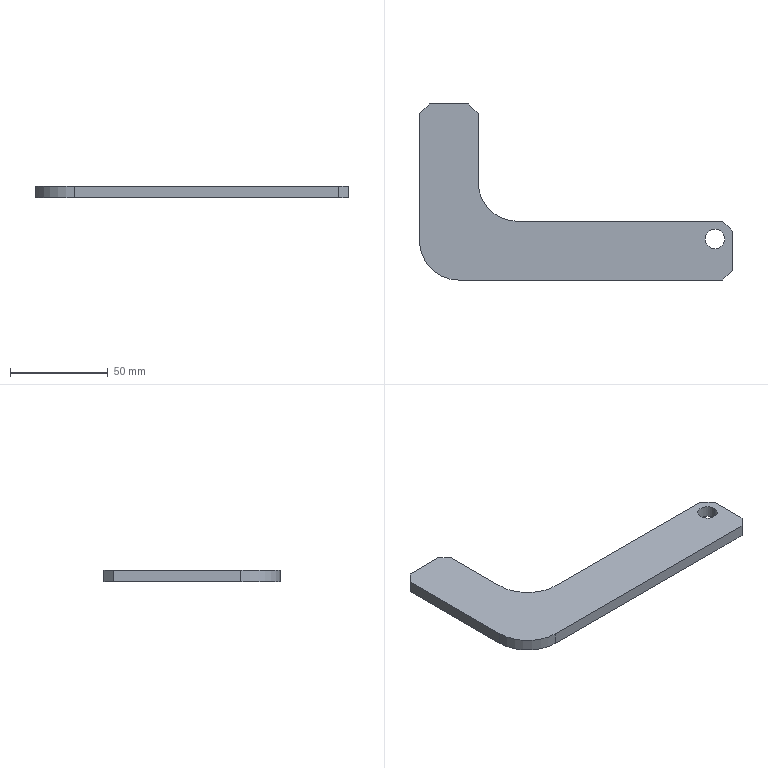Part | STEP file | [02]-12 | 1 solid | 16 faces | box 160 x 90 x 6 mm | volume 38829 mm3 | plane 12 | cylinder 4 | commonest cylinder face diameters 10 x2 40 x2
STEP:
#1=CARTESIAN_POINT('',(146.,21.,6.));
#2=VERTEX_POINT('',#1);
#3=CARTESIAN_POINT('',(156.,21.,6.));
#4=VERTEX_POINT('',#3);
#5=CARTESIAN_POINT('',(151.,21.,6.));
#6=DIRECTION('',(0.,0.,-1.));
#7=DIRECTION('',(1.,0.,0.));
#8=AXIS2_PLACEMENT_3D('',#5,#6,#7);
#9=CIRCLE('',#8,5.);
#10=EDGE_CURVE('',#2,#4,#9,.T.);
#11=ORIENTED_EDGE('',*,*,#10,.F.);
#12=CARTESIAN_POINT('',(146.,21.,0.));
#13=VERTEX_POINT('',#12);
#14=CARTESIAN_POINT('',(146.,21.,6.));
#15=DIRECTION('',(0.,0.,-1.));
#16=VECTOR('',#15,1000.);
#17=LINE('',#14,#16);
#18=EDGE_CURVE('',#2,#13,#17,.T.);
#19=ORIENTED_EDGE('',*,*,#18,.T.);
#20=CARTESIAN_POINT('',(156.,21.,0.));
#21=VERTEX_POINT('',#20);
#22=CARTESIAN_POINT('',(151.,21.,0.));
#23=DIRECTION('',(0.,0.,1.));
#24=DIRECTION('',(-1.,0.,0.));
#25=AXIS2_PLACEMENT_3D('',#22,#23,#24);
#26=CIRCLE('',#25,5.);
#27=EDGE_CURVE('',#21,#13,#26,.T.);
#28=ORIENTED_EDGE('',*,*,#27,.F.);
#29=CARTESIAN_POINT('',(156.,21.,6.));
#30=DIRECTION('',(0.,0.,-1.));
#31=VECTOR('',#30,1000.);
#32=LINE('',#29,#31);
#33=EDGE_CURVE('',#4,#21,#32,.T.);
#34=ORIENTED_EDGE('',*,*,#33,.F.);
#35=EDGE_LOOP('',(#11,#19,#28,#34));
#36=FACE_OUTER_BOUND('',#35,.T.);
#37=CARTESIAN_POINT('',(151.,21.,6.));
#38=DIRECTION('',(0.,0.,-1.));
#39=DIRECTION('',(1.,0.,0.));
#40=AXIS2_PLACEMENT_3D('',#37,#38,#39);
#41=CYLINDRICAL_SURFACE('',#40,5.);
#42=ADVANCED_FACE('',(#36),#41,.F.);
#43=CARTESIAN_POINT('',(50.,30.,6.));
#44=VERTEX_POINT('',#43);
#45=CARTESIAN_POINT('',(155.,30.,6.));
#46=VERTEX_POINT('',#45);
#47=CARTESIAN_POINT('',(80.,30.,6.));
#48=DIRECTION('',(1.,0.,0.));
#49=VECTOR('',#48,1000.);
#50=LINE('',#47,#49);
#51=EDGE_CURVE('',#44,#46,#50,.T.);
#52=ORIENTED_EDGE('',*,*,#51,.T.);
#53=CARTESIAN_POINT('',(155.,30.,0.));
#54=VERTEX_POINT('',#53);
#55=CARTESIAN_POINT('',(155.,30.,0.));
#56=DIRECTION('',(0.,0.,-1.));
#57=VECTOR('',#56,1000.);
#58=LINE('',#55,#57);
#59=EDGE_CURVE('',#46,#54,#58,.T.);
#60=ORIENTED_EDGE('',*,*,#59,.T.);
#61=CARTESIAN_POINT('',(50.,30.,0.));
#62=VERTEX_POINT('',#61);
#63=CARTESIAN_POINT('',(80.,30.,0.));
#64=DIRECTION('',(-1.,0.,0.));
#65=VECTOR('',#64,1000.);
#66=LINE('',#63,#65);
#67=EDGE_CURVE('',#54,#62,#66,.T.);
#68=ORIENTED_EDGE('',*,*,#67,.T.);
#69=CARTESIAN_POINT('',(50.,30.,6.));
#70=DIRECTION('',(0.,0.,1.));
#71=VECTOR('',#70,1000.);
#72=LINE('',#69,#71);
#73=EDGE_CURVE('',#62,#44,#72,.T.);
#74=ORIENTED_EDGE('',*,*,#73,.T.);
#75=EDGE_LOOP('',(#52,#60,#68,#74));
#76=FACE_OUTER_BOUND('',#75,.T.);
#77=CARTESIAN_POINT('',(80.,30.,0.));
#78=DIRECTION('',(0.,1.,0.));
#79=DIRECTION('',(0.,0.,1.));
#80=AXIS2_PLACEMENT_3D('',#77,#78,#79);
#81=PLANE('',#80);
#82=ADVANCED_FACE('',(#76),#81,.T.);
#83=CARTESIAN_POINT('',(151.,21.,6.));
#84=DIRECTION('',(0.,0.,-1.));
#85=DIRECTION('',(1.,0.,0.));
#86=AXIS2_PLACEMENT_3D('',#83,#84,#85);
#87=CIRCLE('',#86,5.);
#88=EDGE_CURVE('',#4,#2,#87,.T.);
#89=ORIENTED_EDGE('',*,*,#88,.T.);
#90=ORIENTED_EDGE('',*,*,#10,.T.);
#91=EDGE_LOOP('',(#89,#90));
#92=FACE_BOUND('',#91,.T.);
#93=CARTESIAN_POINT('',(0.,20.,6.));
#94=VERTEX_POINT('',#93);
#95=CARTESIAN_POINT('',(0.,85.,6.));
#96=VERTEX_POINT('',#95);
#97=CARTESIAN_POINT('',(0.,15.,6.));
#98=DIRECTION('',(0.,1.,0.));
#99=VECTOR('',#98,1000.);
#100=LINE('',#97,#99);
#101=EDGE_CURVE('',#94,#96,#100,.T.);
#102=ORIENTED_EDGE('',*,*,#101,.F.);
#103=CARTESIAN_POINT('',(20.,0.,6.));
#104=VERTEX_POINT('',#103);
#105=CARTESIAN_POINT('',(20.,20.,6.));
#106=DIRECTION('',(0.,0.,1.));
#107=DIRECTION('',(0.,-1.,0.));
#108=AXIS2_PLACEMENT_3D('',#105,#106,#107);
#109=CIRCLE('',#108,20.);
#110=EDGE_CURVE('',#94,#104,#109,.T.);
#111=ORIENTED_EDGE('',*,*,#110,.T.);
#112=CARTESIAN_POINT('',(155.,0.,6.));
#113=VERTEX_POINT('',#112);
#114=CARTESIAN_POINT('',(80.,0.,6.));
#115=DIRECTION('',(-1.,0.,0.));
#116=VECTOR('',#115,1000.);
#117=LINE('',#114,#116);
#118=EDGE_CURVE('',#113,#104,#117,.T.);
#119=ORIENTED_EDGE('',*,*,#118,.F.);
#120=CARTESIAN_POINT('',(160.,5.,6.));
#121=VERTEX_POINT('',#120);
#122=CARTESIAN_POINT('',(125.,-30.,6.));
#123=DIRECTION('',(0.7071,0.7071,0.));
#124=VECTOR('',#123,1000.);
#125=LINE('',#122,#124);
#126=EDGE_CURVE('',#113,#121,#125,.T.);
#127=ORIENTED_EDGE('',*,*,#126,.T.);
#128=CARTESIAN_POINT('',(160.,25.,6.));
#129=VERTEX_POINT('',#128);
#130=CARTESIAN_POINT('',(160.,15.,6.));
#131=DIRECTION('',(0.,-1.,0.));
#132=VECTOR('',#131,1000.);
#133=LINE('',#130,#132);
#134=EDGE_CURVE('',#129,#121,#133,.T.);
#135=ORIENTED_EDGE('',*,*,#134,.F.);
#136=CARTESIAN_POINT('',(125.,60.,6.));
#137=DIRECTION('',(-0.7071,0.7071,0.));
#138=VECTOR('',#137,1000.);
#139=LINE('',#136,#138);
#140=EDGE_CURVE('',#129,#46,#139,.T.);
#141=ORIENTED_EDGE('',*,*,#140,.T.);
#142=ORIENTED_EDGE('',*,*,#51,.F.);
#143=CARTESIAN_POINT('',(30.,50.,6.));
#144=VERTEX_POINT('',#143);
#145=CARTESIAN_POINT('',(50.,50.,6.));
#146=DIRECTION('',(0.,0.,-1.));
#147=DIRECTION('',(0.,-1.,0.));
#148=AXIS2_PLACEMENT_3D('',#145,#146,#147);
#149=CIRCLE('',#148,20.);
#150=EDGE_CURVE('',#44,#144,#149,.T.);
#151=ORIENTED_EDGE('',*,*,#150,.T.);
#152=CARTESIAN_POINT('',(30.,85.,6.));
#153=VERTEX_POINT('',#152);
#154=CARTESIAN_POINT('',(30.,60.,6.));
#155=DIRECTION('',(0.,-1.,0.));
#156=VECTOR('',#155,1000.);
#157=LINE('',#154,#156);
#158=EDGE_CURVE('',#153,#144,#157,.T.);
#159=ORIENTED_EDGE('',*,*,#158,.F.);
#160=CARTESIAN_POINT('',(25.,90.,6.));
#161=VERTEX_POINT('',#160);
#162=CARTESIAN_POINT('',(90.,25.,6.));
#163=DIRECTION('',(-0.7071,0.7071,0.));
#164=VECTOR('',#163,1000.);
#165=LINE('',#162,#164);
#166=EDGE_CURVE('',#153,#161,#165,.T.);
#167=ORIENTED_EDGE('',*,*,#166,.T.);
#168=CARTESIAN_POINT('',(5.,90.,6.));
#169=VERTEX_POINT('',#168);
#170=CARTESIAN_POINT('',(15.,90.,6.));
#171=DIRECTION('',(1.,0.,0.));
#172=VECTOR('',#171,1000.);
#173=LINE('',#170,#172);
#174=EDGE_CURVE('',#169,#161,#173,.T.);
#175=ORIENTED_EDGE('',*,*,#174,.F.);
#176=CARTESIAN_POINT('',(5.,90.,6.));
#177=DIRECTION('',(-0.7071,-0.7071,0.));
#178=VECTOR('',#177,1000.);
#179=LINE('',#176,#178);
#180=EDGE_CURVE('',#169,#96,#179,.T.);
#181=ORIENTED_EDGE('',*,*,#180,.T.);
#182=EDGE_LOOP('',(#102,#111,#119,#127,#135,#141,#142,#151,#159,#167,#175,#181));
#183=FACE_OUTER_BOUND('',#182,.T.);
#184=CARTESIAN_POINT('',(80.,15.,6.));
#185=DIRECTION('',(0.,0.,1.));
#186=DIRECTION('',(0.,-1.,0.));
#187=AXIS2_PLACEMENT_3D('',#184,#185,#186);
#188=PLANE('',#187);
#189=ADVANCED_FACE('',(#92,#183),#188,.T.);
#190=CARTESIAN_POINT('',(0.,85.,0.));
#191=VERTEX_POINT('',#190);
#192=CARTESIAN_POINT('',(0.,20.,0.));
#193=VERTEX_POINT('',#192);
#194=CARTESIAN_POINT('',(0.,15.,0.));
#195=DIRECTION('',(0.,-1.,0.));
#196=VECTOR('',#195,1000.);
#197=LINE('',#194,#196);
#198=EDGE_CURVE('',#191,#193,#197,.T.);
#199=ORIENTED_EDGE('',*,*,#198,.T.);
#200=CARTESIAN_POINT('',(0.,20.,0.));
#201=DIRECTION('',(0.,0.,1.));
#202=VECTOR('',#201,1000.);
#203=LINE('',#200,#202);
#204=EDGE_CURVE('',#193,#94,#203,.T.);
#205=ORIENTED_EDGE('',*,*,#204,.T.);
#206=ORIENTED_EDGE('',*,*,#101,.T.);
#207=CARTESIAN_POINT('',(0.,85.,0.));
#208=DIRECTION('',(0.,0.,-1.));
#209=VECTOR('',#208,1000.);
#210=LINE('',#207,#209);
#211=EDGE_CURVE('',#96,#191,#210,.T.);
#212=ORIENTED_EDGE('',*,*,#211,.T.);
#213=EDGE_LOOP('',(#199,#205,#206,#212));
#214=FACE_OUTER_BOUND('',#213,.T.);
#215=CARTESIAN_POINT('',(0.,15.,0.));
#216=DIRECTION('',(-1.,0.,0.));
#217=DIRECTION('',(0.,0.,-1.));
#218=AXIS2_PLACEMENT_3D('',#215,#216,#217);
#219=PLANE('',#218);
#220=ADVANCED_FACE('',(#214),#219,.T.);
#221=CARTESIAN_POINT('',(160.,5.,0.));
#222=VERTEX_POINT('',#221);
#223=CARTESIAN_POINT('',(160.,25.,0.));
#224=VERTEX_POINT('',#223);
#225=CARTESIAN_POINT('',(160.,15.,0.));
#226=DIRECTION('',(0.,1.,0.));
#227=VECTOR('',#226,1000.);
#228=LINE('',#225,#227);
#229=EDGE_CURVE('',#222,#224,#228,.T.);
#230=ORIENTED_EDGE('',*,*,#229,.T.);
#231=CARTESIAN_POINT('',(160.,25.,0.));
#232=DIRECTION('',(0.,0.,1.));
#233=VECTOR('',#232,1000.);
#234=LINE('',#231,#233);
#235=EDGE_CURVE('',#224,#129,#234,.T.);
#236=ORIENTED_EDGE('',*,*,#235,.T.);
#237=ORIENTED_EDGE('',*,*,#134,.T.);
#238=CARTESIAN_POINT('',(160.,5.,0.));
#239=DIRECTION('',(0.,0.,-1.));
#240=VECTOR('',#239,1000.);
#241=LINE('',#238,#240);
#242=EDGE_CURVE('',#121,#222,#241,.T.);
#243=ORIENTED_EDGE('',*,*,#242,.T.);
#244=EDGE_LOOP('',(#230,#236,#237,#243));
#245=FACE_OUTER_BOUND('',#244,.T.);
#246=CARTESIAN_POINT('',(160.,15.,0.));
#247=DIRECTION('',(1.,0.,0.));
#248=DIRECTION('',(0.,0.,1.));
#249=AXIS2_PLACEMENT_3D('',#246,#247,#248);
#250=PLANE('',#249);
#251=ADVANCED_FACE('',(#245),#250,.T.);
#252=ORIENTED_EDGE('',*,*,#27,.T.);
#253=CARTESIAN_POINT('',(151.,21.,0.));
#254=DIRECTION('',(0.,0.,1.));
#255=DIRECTION('',(-1.,0.,0.));
#256=AXIS2_PLACEMENT_3D('',#253,#254,#255);
#257=CIRCLE('',#256,5.);
#258=EDGE_CURVE('',#13,#21,#257,.T.);
#259=ORIENTED_EDGE('',*,*,#258,.T.);
#260=EDGE_LOOP('',(#252,#259));
#261=FACE_BOUND('',#260,.T.);
#262=CARTESIAN_POINT('',(20.,0.,0.));
#263=VERTEX_POINT('',#262);
#264=CARTESIAN_POINT('',(155.,0.,0.));
#265=VERTEX_POINT('',#264);
#266=CARTESIAN_POINT('',(80.,0.,0.));
#267=DIRECTION('',(1.,0.,0.));
#268=VECTOR('',#267,1000.);
#269=LINE('',#266,#268);
#270=EDGE_CURVE('',#263,#265,#269,.T.);
#271=ORIENTED_EDGE('',*,*,#270,.F.);
#272=CARTESIAN_POINT('',(20.,20.,0.));
#273=DIRECTION('',(0.,0.,-1.));
#274=DIRECTION('',(0.,1.,0.));
#275=AXIS2_PLACEMENT_3D('',#272,#273,#274);
#276=CIRCLE('',#275,20.);
#277=EDGE_CURVE('',#263,#193,#276,.T.);
#278=ORIENTED_EDGE('',*,*,#277,.T.);
#279=ORIENTED_EDGE('',*,*,#198,.F.);
#280=CARTESIAN_POINT('',(5.,90.,0.));
#281=VERTEX_POINT('',#280);
#282=CARTESIAN_POINT('',(5.,90.,0.));
#283=DIRECTION('',(0.7071,0.7071,0.));
#284=VECTOR('',#283,1000.);
#285=LINE('',#282,#284);
#286=EDGE_CURVE('',#191,#281,#285,.T.);
#287=ORIENTED_EDGE('',*,*,#286,.T.);
#288=CARTESIAN_POINT('',(25.,90.,0.));
#289=VERTEX_POINT('',#288);
#290=CARTESIAN_POINT('',(15.,90.,0.));
#291=DIRECTION('',(-1.,0.,0.));
#292=VECTOR('',#291,1000.);
#293=LINE('',#290,#292);
#294=EDGE_CURVE('',#289,#281,#293,.T.);
#295=ORIENTED_EDGE('',*,*,#294,.F.);
#296=CARTESIAN_POINT('',(30.,85.,0.));
#297=VERTEX_POINT('',#296);
#298=CARTESIAN_POINT('',(90.,25.,0.));
#299=DIRECTION('',(0.7071,-0.7071,0.));
#300=VECTOR('',#299,1000.);
#301=LINE('',#298,#300);
#302=EDGE_CURVE('',#289,#297,#301,.T.);
#303=ORIENTED_EDGE('',*,*,#302,.T.);
#304=CARTESIAN_POINT('',(30.,50.,0.));
#305=VERTEX_POINT('',#304);
#306=CARTESIAN_POINT('',(30.,60.,0.));
#307=DIRECTION('',(0.,1.,0.));
#308=VECTOR('',#307,1000.);
#309=LINE('',#306,#308);
#310=EDGE_CURVE('',#305,#297,#309,.T.);
#311=ORIENTED_EDGE('',*,*,#310,.F.);
#312=CARTESIAN_POINT('',(50.,50.,0.));
#313=DIRECTION('',(0.,0.,1.));
#314=DIRECTION('',(0.,1.,0.));
#315=AXIS2_PLACEMENT_3D('',#312,#313,#314);
#316=CIRCLE('',#315,20.);
#317=EDGE_CURVE('',#305,#62,#316,.T.);
#318=ORIENTED_EDGE('',*,*,#317,.T.);
#319=ORIENTED_EDGE('',*,*,#67,.F.);
#320=CARTESIAN_POINT('',(125.,60.,0.));
#321=DIRECTION('',(0.7071,-0.7071,0.));
#322=VECTOR('',#321,1000.);
#323=LINE('',#320,#322);
#324=EDGE_CURVE('',#54,#224,#323,.T.);
#325=ORIENTED_EDGE('',*,*,#324,.T.);
#326=ORIENTED_EDGE('',*,*,#229,.F.);
#327=CARTESIAN_POINT('',(125.,-30.,0.));
#328=DIRECTION('',(-0.7071,-0.7071,0.));
#329=VECTOR('',#328,1000.);
#330=LINE('',#327,#329);
#331=EDGE_CURVE('',#222,#265,#330,.T.);
#332=ORIENTED_EDGE('',*,*,#331,.T.);
#333=EDGE_LOOP('',(#271,#278,#279,#287,#295,#303,#311,#318,#319,#325,#326,#332));
#334=FACE_OUTER_BOUND('',#333,.T.);
#335=CARTESIAN_POINT('',(80.,15.,0.));
#336=DIRECTION('',(0.,0.,-1.));
#337=DIRECTION('',(0.,1.,0.));
#338=AXIS2_PLACEMENT_3D('',#335,#336,#337);
#339=PLANE('',#338);
#340=ADVANCED_FACE('',(#261,#334),#339,.T.);
#341=ORIENTED_EDGE('',*,*,#118,.T.);
#342=CARTESIAN_POINT('',(20.,0.,0.));
#343=DIRECTION('',(0.,0.,-1.));
#344=VECTOR('',#343,1000.);
#345=LINE('',#342,#344);
#346=EDGE_CURVE('',#104,#263,#345,.T.);
#347=ORIENTED_EDGE('',*,*,#346,.T.);
#348=ORIENTED_EDGE('',*,*,#270,.T.);
#349=CARTESIAN_POINT('',(155.,0.,0.));
#350=DIRECTION('',(0.,0.,1.));
#351=VECTOR('',#350,1000.);
#352=LINE('',#349,#351);
#353=EDGE_CURVE('',#265,#113,#352,.T.);
#354=ORIENTED_EDGE('',*,*,#353,.T.);
#355=EDGE_LOOP('',(#341,#347,#348,#354));
#356=FACE_OUTER_BOUND('',#355,.T.);
#357=CARTESIAN_POINT('',(80.,0.,0.));
#358=DIRECTION('',(0.,-1.,0.));
#359=DIRECTION('',(0.,0.,-1.));
#360=AXIS2_PLACEMENT_3D('',#357,#358,#359);
#361=PLANE('',#360);
#362=ADVANCED_FACE('',(#356),#361,.T.);
#363=ORIENTED_EDGE('',*,*,#294,.T.);
#364=CARTESIAN_POINT('',(5.,90.,0.));
#365=DIRECTION('',(0.,0.,1.));
#366=VECTOR('',#365,1000.);
#367=LINE('',#364,#366);
#368=EDGE_CURVE('',#281,#169,#367,.T.);
#369=ORIENTED_EDGE('',*,*,#368,.T.);
#370=ORIENTED_EDGE('',*,*,#174,.T.);
#371=CARTESIAN_POINT('',(25.,90.,0.));
#372=DIRECTION('',(0.,0.,-1.));
#373=VECTOR('',#372,1000.);
#374=LINE('',#371,#373);
#375=EDGE_CURVE('',#161,#289,#374,.T.);
#376=ORIENTED_EDGE('',*,*,#375,.T.);
#377=EDGE_LOOP('',(#363,#369,#370,#376));
#378=FACE_OUTER_BOUND('',#377,.T.);
#379=CARTESIAN_POINT('',(15.,90.,0.));
#380=DIRECTION('',(0.,1.,0.));
#381=DIRECTION('',(0.,0.,1.));
#382=AXIS2_PLACEMENT_3D('',#379,#380,#381);
#383=PLANE('',#382);
#384=ADVANCED_FACE('',(#378),#383,.T.);
#385=ORIENTED_EDGE('',*,*,#310,.T.);
#386=CARTESIAN_POINT('',(30.,85.,0.));
#387=DIRECTION('',(0.,0.,1.));
#388=VECTOR('',#387,1000.);
#389=LINE('',#386,#388);
#390=EDGE_CURVE('',#297,#153,#389,.T.);
#391=ORIENTED_EDGE('',*,*,#390,.T.);
#392=ORIENTED_EDGE('',*,*,#158,.T.);
#393=CARTESIAN_POINT('',(30.,50.,0.));
#394=DIRECTION('',(0.,0.,-1.));
#395=VECTOR('',#394,1000.);
#396=LINE('',#393,#395);
#397=EDGE_CURVE('',#144,#305,#396,.T.);
#398=ORIENTED_EDGE('',*,*,#397,.T.);
#399=EDGE_LOOP('',(#385,#391,#392,#398));
#400=FACE_OUTER_BOUND('',#399,.T.);
#401=CARTESIAN_POINT('',(30.,60.,0.));
#402=DIRECTION('',(1.,0.,0.));
#403=DIRECTION('',(0.,0.,1.));
#404=AXIS2_PLACEMENT_3D('',#401,#402,#403);
#405=PLANE('',#404);
#406=ADVANCED_FACE('',(#400),#405,.T.);
#407=ORIENTED_EDGE('',*,*,#317,.F.);
#408=ORIENTED_EDGE('',*,*,#397,.F.);
#409=ORIENTED_EDGE('',*,*,#150,.F.);
#410=ORIENTED_EDGE('',*,*,#73,.F.);
#411=EDGE_LOOP('',(#407,#408,#409,#410));
#412=FACE_OUTER_BOUND('',#411,.T.);
#413=CARTESIAN_POINT('',(50.,50.,0.));
#414=DIRECTION('',(0.,0.,-1.));
#415=DIRECTION('',(0.,1.,0.));
#416=AXIS2_PLACEMENT_3D('',#413,#414,#415);
#417=CYLINDRICAL_SURFACE('',#416,20.);
#418=ADVANCED_FACE('',(#412),#417,.F.);
#419=ORIENTED_EDGE('',*,*,#302,.F.);
#420=ORIENTED_EDGE('',*,*,#375,.F.);
#421=ORIENTED_EDGE('',*,*,#166,.F.);
#422=ORIENTED_EDGE('',*,*,#390,.F.);
#423=EDGE_LOOP('',(#419,#420,#421,#422));
#424=FACE_OUTER_BOUND('',#423,.T.);
#425=CARTESIAN_POINT('',(30.,85.,0.));
#426=DIRECTION('',(-0.7071,-0.7071,0.));
#427=DIRECTION('',(0.,0.,1.));
#428=AXIS2_PLACEMENT_3D('',#425,#426,#427);
#429=PLANE('',#428);
#430=ADVANCED_FACE('',(#424),#429,.F.);
#431=ORIENTED_EDGE('',*,*,#286,.F.);
#432=ORIENTED_EDGE('',*,*,#211,.F.);
#433=ORIENTED_EDGE('',*,*,#180,.F.);
#434=ORIENTED_EDGE('',*,*,#368,.F.);
#435=EDGE_LOOP('',(#431,#432,#433,#434));
#436=FACE_OUTER_BOUND('',#435,.T.);
#437=CARTESIAN_POINT('',(5.,90.,0.));
#438=DIRECTION('',(0.7071,-0.7071,0.));
#439=DIRECTION('',(0.,0.,1.));
#440=AXIS2_PLACEMENT_3D('',#437,#438,#439);
#441=PLANE('',#440);
#442=ADVANCED_FACE('',(#436),#441,.F.);
#443=ORIENTED_EDGE('',*,*,#331,.F.);
#444=ORIENTED_EDGE('',*,*,#242,.F.);
#445=ORIENTED_EDGE('',*,*,#126,.F.);
#446=ORIENTED_EDGE('',*,*,#353,.F.);
#447=EDGE_LOOP('',(#443,#444,#445,#446));
#448=FACE_OUTER_BOUND('',#447,.T.);
#449=CARTESIAN_POINT('',(155.,0.,0.));
#450=DIRECTION('',(-0.7071,0.7071,0.));
#451=DIRECTION('',(0.,0.,1.));
#452=AXIS2_PLACEMENT_3D('',#449,#450,#451);
#453=PLANE('',#452);
#454=ADVANCED_FACE('',(#448),#453,.F.);
#455=ORIENTED_EDGE('',*,*,#324,.F.);
#456=ORIENTED_EDGE('',*,*,#59,.F.);
#457=ORIENTED_EDGE('',*,*,#140,.F.);
#458=ORIENTED_EDGE('',*,*,#235,.F.);
#459=EDGE_LOOP('',(#455,#456,#457,#458));
#460=FACE_OUTER_BOUND('',#459,.T.);
#461=CARTESIAN_POINT('',(160.,25.,0.));
#462=DIRECTION('',(-0.7071,-0.7071,0.));
#463=DIRECTION('',(0.,0.,1.));
#464=AXIS2_PLACEMENT_3D('',#461,#462,#463);
#465=PLANE('',#464);
#466=ADVANCED_FACE('',(#460),#465,.F.);
#467=ORIENTED_EDGE('',*,*,#277,.F.);
#468=ORIENTED_EDGE('',*,*,#346,.F.);
#469=ORIENTED_EDGE('',*,*,#110,.F.);
#470=ORIENTED_EDGE('',*,*,#204,.F.);
#471=EDGE_LOOP('',(#467,#468,#469,#470));
#472=FACE_OUTER_BOUND('',#471,.T.);
#473=CARTESIAN_POINT('',(20.,20.,0.));
#474=DIRECTION('',(0.,0.,1.));
#475=DIRECTION('',(0.,-1.,0.));
#476=AXIS2_PLACEMENT_3D('',#473,#474,#475);
#477=CYLINDRICAL_SURFACE('',#476,20.);
#478=ADVANCED_FACE('',(#472),#477,.T.);
#479=ORIENTED_EDGE('',*,*,#18,.F.);
#480=ORIENTED_EDGE('',*,*,#88,.F.);
#481=ORIENTED_EDGE('',*,*,#33,.T.);
#482=ORIENTED_EDGE('',*,*,#258,.F.);
#483=EDGE_LOOP('',(#479,#480,#481,#482));
#484=FACE_OUTER_BOUND('',#483,.T.);
#485=CARTESIAN_POINT('',(151.,21.,6.));
#486=DIRECTION('',(0.,0.,-1.));
#487=DIRECTION('',(1.,0.,0.));
#488=AXIS2_PLACEMENT_3D('',#485,#486,#487);
#489=CYLINDRICAL_SURFACE('',#488,5.);
#490=ADVANCED_FACE('',(#484),#489,.F.);
#491=CLOSED_SHELL('',(#42,#82,#189,#220,#251,#340,#362,#384,#406,#418,#430,#442,#454,#466,#478,#490));
#492=MANIFOLD_SOLID_BREP('',#491);
#493=CARTESIAN_POINT('',(0.,0.,0.));
#494=DIRECTION('',(0.,0.,1.));
#495=DIRECTION('',(1.,0.,0.));
#496=AXIS2_PLACEMENT_3D('',#493,#494,#495);
#497=(LENGTH_UNIT()NAMED_UNIT(*)SI_UNIT(.MILLI.,.METRE.));
#498=UNCERTAINTY_MEASURE_WITH_UNIT(LENGTH_MEASURE(0.00001),#497,'','');
#499=(NAMED_UNIT(*)PLANE_ANGLE_UNIT()SI_UNIT($,.RADIAN.));
#500=(NAMED_UNIT(*)SI_UNIT($,.STERADIAN.)SOLID_ANGLE_UNIT());
#501=(GEOMETRIC_REPRESENTATION_CONTEXT(3)GLOBAL_UNCERTAINTY_ASSIGNED_CONTEXT((#498))GLOBAL_UNIT_ASSIGNED_CONTEXT((#497,#499,#500))REPRESENTATION_CONTEXT('',''));
#502=ADVANCED_BREP_SHAPE_REPRESENTATION('',(#492,#496),#501);